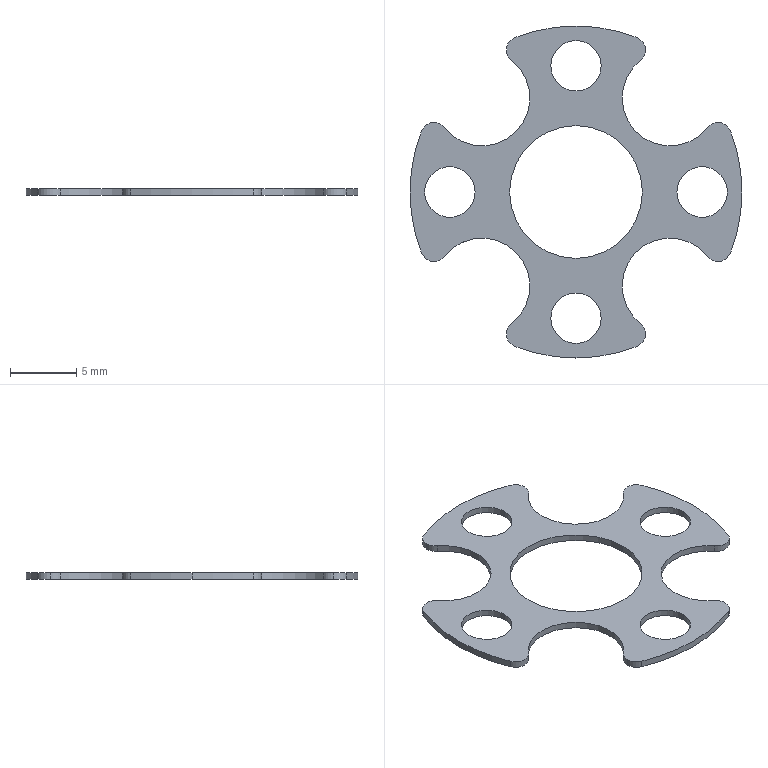Part | SolidWorks | features Extrusion 1 | 1 solid | 33 faces | box 25 x 25 x 0.5 mm | volume 107.561 mm3 | cylinder 31 | plane 2 | commonest cylinder face diameters 2 x10 3.8 x8 7.2 x6 25 x5 10 x2
STEP:
#1=CARTESIAN_POINT('',(-11.4,0.,0.5));
#2=VERTEX_POINT('',#1);
#3=CARTESIAN_POINT('',(-7.6,0.,0.5));
#4=VERTEX_POINT('',#3);
#5=CARTESIAN_POINT('',(-9.5,0.,0.5));
#6=DIRECTION('',(0.,0.,1.));
#7=DIRECTION('',(1.,0.,0.));
#8=AXIS2_PLACEMENT_3D('',#5,#6,#7);
#9=CIRCLE('',#8,1.9);
#10=EDGE_CURVE('',#2,#4,#9,.T.);
#11=ORIENTED_EDGE('',*,*,#10,.T.);
#12=CARTESIAN_POINT('',(-7.6,0.,0.));
#13=VERTEX_POINT('',#12);
#14=CARTESIAN_POINT('',(-7.6,0.,0.5));
#15=DIRECTION('',(0.,0.,-1.));
#16=VECTOR('',#15,1000.);
#17=LINE('',#14,#16);
#18=EDGE_CURVE('',#4,#13,#17,.T.);
#19=ORIENTED_EDGE('',*,*,#18,.T.);
#20=CARTESIAN_POINT('',(-11.4,0.,0.));
#21=VERTEX_POINT('',#20);
#22=CARTESIAN_POINT('',(-9.5,0.,0.));
#23=DIRECTION('',(0.,0.,1.));
#24=DIRECTION('',(1.,0.,0.));
#25=AXIS2_PLACEMENT_3D('',#22,#23,#24);
#26=CIRCLE('',#25,1.9);
#27=EDGE_CURVE('',#21,#13,#26,.T.);
#28=ORIENTED_EDGE('',*,*,#27,.F.);
#29=CARTESIAN_POINT('',(-11.4,0.,0.5));
#30=DIRECTION('',(0.,0.,-1.));
#31=VECTOR('',#30,1000.);
#32=LINE('',#29,#31);
#33=EDGE_CURVE('',#2,#21,#32,.T.);
#34=ORIENTED_EDGE('',*,*,#33,.F.);
#35=EDGE_LOOP('',(#11,#19,#28,#34));
#36=FACE_OUTER_BOUND('',#35,.T.);
#37=CARTESIAN_POINT('',(-9.5,0.,0.5));
#38=DIRECTION('',(0.,0.,-1.));
#39=DIRECTION('',(-1.,0.,0.));
#40=AXIS2_PLACEMENT_3D('',#37,#38,#39);
#41=CYLINDRICAL_SURFACE('',#40,1.9);
#42=ADVANCED_FACE('',(#36),#41,.F.);
#43=CARTESIAN_POINT('',(-1.9,-9.5,0.5));
#44=VERTEX_POINT('',#43);
#45=CARTESIAN_POINT('',(1.9,-9.5,0.5));
#46=VERTEX_POINT('',#45);
#47=CARTESIAN_POINT('',(0.,-9.5,0.5));
#48=DIRECTION('',(0.,0.,1.));
#49=DIRECTION('',(1.,0.,0.));
#50=AXIS2_PLACEMENT_3D('',#47,#48,#49);
#51=CIRCLE('',#50,1.9);
#52=EDGE_CURVE('',#44,#46,#51,.T.);
#53=ORIENTED_EDGE('',*,*,#52,.T.);
#54=CARTESIAN_POINT('',(1.9,-9.5,0.));
#55=VERTEX_POINT('',#54);
#56=CARTESIAN_POINT('',(1.9,-9.5,0.5));
#57=DIRECTION('',(0.,0.,-1.));
#58=VECTOR('',#57,1000.);
#59=LINE('',#56,#58);
#60=EDGE_CURVE('',#46,#55,#59,.T.);
#61=ORIENTED_EDGE('',*,*,#60,.T.);
#62=CARTESIAN_POINT('',(-1.9,-9.5,0.));
#63=VERTEX_POINT('',#62);
#64=CARTESIAN_POINT('',(0.,-9.5,0.));
#65=DIRECTION('',(0.,0.,1.));
#66=DIRECTION('',(1.,0.,0.));
#67=AXIS2_PLACEMENT_3D('',#64,#65,#66);
#68=CIRCLE('',#67,1.9);
#69=EDGE_CURVE('',#63,#55,#68,.T.);
#70=ORIENTED_EDGE('',*,*,#69,.F.);
#71=CARTESIAN_POINT('',(-1.9,-9.5,0.5));
#72=DIRECTION('',(0.,0.,-1.));
#73=VECTOR('',#72,1000.);
#74=LINE('',#71,#73);
#75=EDGE_CURVE('',#44,#63,#74,.T.);
#76=ORIENTED_EDGE('',*,*,#75,.F.);
#77=EDGE_LOOP('',(#53,#61,#70,#76));
#78=FACE_OUTER_BOUND('',#77,.T.);
#79=CARTESIAN_POINT('',(0.,-9.5,0.5));
#80=DIRECTION('',(0.,0.,-1.));
#81=DIRECTION('',(-1.,0.,0.));
#82=AXIS2_PLACEMENT_3D('',#79,#80,#81);
#83=CYLINDRICAL_SURFACE('',#82,1.9);
#84=ADVANCED_FACE('',(#78),#83,.F.);
#85=CARTESIAN_POINT('',(7.6,0.,0.5));
#86=VERTEX_POINT('',#85);
#87=CARTESIAN_POINT('',(11.4,0.,0.5));
#88=VERTEX_POINT('',#87);
#89=CARTESIAN_POINT('',(9.5,0.,0.5));
#90=DIRECTION('',(0.,0.,1.));
#91=DIRECTION('',(1.,0.,0.));
#92=AXIS2_PLACEMENT_3D('',#89,#90,#91);
#93=CIRCLE('',#92,1.9);
#94=EDGE_CURVE('',#86,#88,#93,.T.);
#95=ORIENTED_EDGE('',*,*,#94,.T.);
#96=CARTESIAN_POINT('',(11.4,0.,0.));
#97=VERTEX_POINT('',#96);
#98=CARTESIAN_POINT('',(11.4,0.,0.5));
#99=DIRECTION('',(0.,0.,-1.));
#100=VECTOR('',#99,1000.);
#101=LINE('',#98,#100);
#102=EDGE_CURVE('',#88,#97,#101,.T.);
#103=ORIENTED_EDGE('',*,*,#102,.T.);
#104=CARTESIAN_POINT('',(7.6,0.,0.));
#105=VERTEX_POINT('',#104);
#106=CARTESIAN_POINT('',(9.5,0.,0.));
#107=DIRECTION('',(0.,0.,1.));
#108=DIRECTION('',(1.,0.,0.));
#109=AXIS2_PLACEMENT_3D('',#106,#107,#108);
#110=CIRCLE('',#109,1.9);
#111=EDGE_CURVE('',#105,#97,#110,.T.);
#112=ORIENTED_EDGE('',*,*,#111,.F.);
#113=CARTESIAN_POINT('',(7.6,0.,0.5));
#114=DIRECTION('',(0.,0.,-1.));
#115=VECTOR('',#114,1000.);
#116=LINE('',#113,#115);
#117=EDGE_CURVE('',#86,#105,#116,.T.);
#118=ORIENTED_EDGE('',*,*,#117,.F.);
#119=EDGE_LOOP('',(#95,#103,#112,#118));
#120=FACE_OUTER_BOUND('',#119,.T.);
#121=CARTESIAN_POINT('',(9.5,0.,0.5));
#122=DIRECTION('',(0.,0.,-1.));
#123=DIRECTION('',(-1.,0.,0.));
#124=AXIS2_PLACEMENT_3D('',#121,#122,#123);
#125=CYLINDRICAL_SURFACE('',#124,1.9);
#126=ADVANCED_FACE('',(#120),#125,.F.);
#127=CARTESIAN_POINT('',(-5.,0.,0.5));
#128=VERTEX_POINT('',#127);
#129=CARTESIAN_POINT('',(5.,0.,0.5));
#130=VERTEX_POINT('',#129);
#131=CARTESIAN_POINT('',(0.,0.,0.5));
#132=DIRECTION('',(0.,0.,1.));
#133=DIRECTION('',(1.,0.,0.));
#134=AXIS2_PLACEMENT_3D('',#131,#132,#133);
#135=CIRCLE('',#134,5.);
#136=EDGE_CURVE('',#128,#130,#135,.T.);
#137=ORIENTED_EDGE('',*,*,#136,.T.);
#138=CARTESIAN_POINT('',(5.,0.,0.));
#139=VERTEX_POINT('',#138);
#140=CARTESIAN_POINT('',(5.,0.,0.5));
#141=DIRECTION('',(0.,0.,-1.));
#142=VECTOR('',#141,1000.);
#143=LINE('',#140,#142);
#144=EDGE_CURVE('',#130,#139,#143,.T.);
#145=ORIENTED_EDGE('',*,*,#144,.T.);
#146=CARTESIAN_POINT('',(-5.,0.,0.));
#147=VERTEX_POINT('',#146);
#148=CARTESIAN_POINT('',(0.,0.,0.));
#149=DIRECTION('',(0.,0.,1.));
#150=DIRECTION('',(1.,0.,0.));
#151=AXIS2_PLACEMENT_3D('',#148,#149,#150);
#152=CIRCLE('',#151,5.);
#153=EDGE_CURVE('',#147,#139,#152,.T.);
#154=ORIENTED_EDGE('',*,*,#153,.F.);
#155=CARTESIAN_POINT('',(-5.,0.,0.5));
#156=DIRECTION('',(0.,0.,-1.));
#157=VECTOR('',#156,1000.);
#158=LINE('',#155,#157);
#159=EDGE_CURVE('',#128,#147,#158,.T.);
#160=ORIENTED_EDGE('',*,*,#159,.F.);
#161=EDGE_LOOP('',(#137,#145,#154,#160));
#162=FACE_OUTER_BOUND('',#161,.T.);
#163=CARTESIAN_POINT('',(0.,0.,0.5));
#164=DIRECTION('',(0.,0.,-1.));
#165=DIRECTION('',(-1.,0.,0.));
#166=AXIS2_PLACEMENT_3D('',#163,#164,#165);
#167=CYLINDRICAL_SURFACE('',#166,5.);
#168=ADVANCED_FACE('',(#162),#167,.F.);
#169=CARTESIAN_POINT('',(-1.9,9.5,0.5));
#170=VERTEX_POINT('',#169);
#171=CARTESIAN_POINT('',(1.9,9.5,0.5));
#172=VERTEX_POINT('',#171);
#173=CARTESIAN_POINT('',(0.,9.5,0.5));
#174=DIRECTION('',(0.,0.,1.));
#175=DIRECTION('',(1.,0.,0.));
#176=AXIS2_PLACEMENT_3D('',#173,#174,#175);
#177=CIRCLE('',#176,1.9);
#178=EDGE_CURVE('',#170,#172,#177,.T.);
#179=ORIENTED_EDGE('',*,*,#178,.T.);
#180=CARTESIAN_POINT('',(1.9,9.5,0.));
#181=VERTEX_POINT('',#180);
#182=CARTESIAN_POINT('',(1.9,9.5,0.5));
#183=DIRECTION('',(0.,0.,-1.));
#184=VECTOR('',#183,1000.);
#185=LINE('',#182,#184);
#186=EDGE_CURVE('',#172,#181,#185,.T.);
#187=ORIENTED_EDGE('',*,*,#186,.T.);
#188=CARTESIAN_POINT('',(-1.9,9.5,0.));
#189=VERTEX_POINT('',#188);
#190=CARTESIAN_POINT('',(0.,9.5,0.));
#191=DIRECTION('',(0.,0.,1.));
#192=DIRECTION('',(1.,0.,0.));
#193=AXIS2_PLACEMENT_3D('',#190,#191,#192);
#194=CIRCLE('',#193,1.9);
#195=EDGE_CURVE('',#189,#181,#194,.T.);
#196=ORIENTED_EDGE('',*,*,#195,.F.);
#197=CARTESIAN_POINT('',(-1.9,9.5,0.5));
#198=DIRECTION('',(0.,0.,-1.));
#199=VECTOR('',#198,1000.);
#200=LINE('',#197,#199);
#201=EDGE_CURVE('',#170,#189,#200,.T.);
#202=ORIENTED_EDGE('',*,*,#201,.F.);
#203=EDGE_LOOP('',(#179,#187,#196,#202));
#204=FACE_OUTER_BOUND('',#203,.T.);
#205=CARTESIAN_POINT('',(0.,9.5,0.5));
#206=DIRECTION('',(0.,0.,-1.));
#207=DIRECTION('',(-1.,0.,0.));
#208=AXIS2_PLACEMENT_3D('',#205,#206,#207);
#209=CYLINDRICAL_SURFACE('',#208,1.9);
#210=ADVANCED_FACE('',(#204),#209,.F.);
#211=CARTESIAN_POINT('',(3.471,-7.071,0.5));
#212=VERTEX_POINT('',#211);
#213=CARTESIAN_POINT('',(9.905,-4.851,0.5));
#214=VERTEX_POINT('',#213);
#215=CARTESIAN_POINT('',(7.071,-7.071,0.5));
#216=DIRECTION('',(0.,0.,-1.));
#217=DIRECTION('',(-1.,0.,0.));
#218=AXIS2_PLACEMENT_3D('',#215,#216,#217);
#219=CIRCLE('',#218,3.6);
#220=EDGE_CURVE('',#212,#214,#219,.T.);
#221=ORIENTED_EDGE('',*,*,#220,.F.);
#222=CARTESIAN_POINT('',(3.471,-7.071,0.));
#223=VERTEX_POINT('',#222);
#224=CARTESIAN_POINT('',(3.471,-7.071,0.5));
#225=DIRECTION('',(0.,0.,-1.));
#226=VECTOR('',#225,1000.);
#227=LINE('',#224,#226);
#228=EDGE_CURVE('',#212,#223,#227,.T.);
#229=ORIENTED_EDGE('',*,*,#228,.T.);
#230=CARTESIAN_POINT('',(9.905,-4.851,0.));
#231=VERTEX_POINT('',#230);
#232=CARTESIAN_POINT('',(7.071,-7.071,0.));
#233=DIRECTION('',(0.,0.,-1.));
#234=DIRECTION('',(-1.,0.,0.));
#235=AXIS2_PLACEMENT_3D('',#232,#233,#234);
#236=CIRCLE('',#235,3.6);
#237=EDGE_CURVE('',#223,#231,#236,.T.);
#238=ORIENTED_EDGE('',*,*,#237,.T.);
#239=CARTESIAN_POINT('',(9.905,-4.851,0.5));
#240=DIRECTION('',(0.,0.,-1.));
#241=VECTOR('',#240,1000.);
#242=LINE('',#239,#241);
#243=EDGE_CURVE('',#214,#231,#242,.T.);
#244=ORIENTED_EDGE('',*,*,#243,.F.);
#245=EDGE_LOOP('',(#221,#229,#238,#244));
#246=FACE_OUTER_BOUND('',#245,.T.);
#247=CARTESIAN_POINT('',(7.071,-7.071,0.5));
#248=DIRECTION('',(0.,0.,-1.));
#249=DIRECTION('',(-1.,0.,0.));
#250=AXIS2_PLACEMENT_3D('',#247,#248,#249);
#251=CYLINDRICAL_SURFACE('',#250,3.6);
#252=ADVANCED_FACE('',(#246),#251,.F.);
#253=CARTESIAN_POINT('',(-5.234,-10.692,0.5));
#254=VERTEX_POINT('',#253);
#255=CARTESIAN_POINT('',(-4.602,-11.622,0.5));
#256=VERTEX_POINT('',#255);
#257=CARTESIAN_POINT('',(-4.234,-10.692,0.5));
#258=DIRECTION('',(0.,0.,1.));
#259=DIRECTION('',(1.,0.,0.));
#260=AXIS2_PLACEMENT_3D('',#257,#258,#259);
#261=CIRCLE('',#260,1.);
#262=EDGE_CURVE('',#254,#256,#261,.T.);
#263=ORIENTED_EDGE('',*,*,#262,.F.);
#264=CARTESIAN_POINT('',(-5.234,-10.692,0.));
#265=VERTEX_POINT('',#264);
#266=CARTESIAN_POINT('',(-5.234,-10.692,0.5));
#267=DIRECTION('',(0.,0.,-1.));
#268=VECTOR('',#267,1000.);
#269=LINE('',#266,#268);
#270=EDGE_CURVE('',#254,#265,#269,.T.);
#271=ORIENTED_EDGE('',*,*,#270,.T.);
#272=CARTESIAN_POINT('',(-4.602,-11.622,0.));
#273=VERTEX_POINT('',#272);
#274=CARTESIAN_POINT('',(-4.234,-10.692,0.));
#275=DIRECTION('',(0.,0.,1.));
#276=DIRECTION('',(1.,0.,0.));
#277=AXIS2_PLACEMENT_3D('',#274,#275,#276);
#278=CIRCLE('',#277,1.);
#279=EDGE_CURVE('',#265,#273,#278,.T.);
#280=ORIENTED_EDGE('',*,*,#279,.T.);
#281=CARTESIAN_POINT('',(-4.602,-11.622,0.5));
#282=DIRECTION('',(0.,0.,-1.));
#283=VECTOR('',#282,1000.);
#284=LINE('',#281,#283);
#285=EDGE_CURVE('',#256,#273,#284,.T.);
#286=ORIENTED_EDGE('',*,*,#285,.F.);
#287=EDGE_LOOP('',(#263,#271,#280,#286));
#288=FACE_OUTER_BOUND('',#287,.T.);
#289=CARTESIAN_POINT('',(-4.234,-10.692,0.5));
#290=DIRECTION('',(0.,0.,-1.));
#291=DIRECTION('',(-1.,0.,0.));
#292=AXIS2_PLACEMENT_3D('',#289,#290,#291);
#293=CYLINDRICAL_SURFACE('',#292,1.);
#294=ADVANCED_FACE('',(#288),#293,.T.);
#295=CARTESIAN_POINT('',(-12.5,0.,0.5));
#296=VERTEX_POINT('',#295);
#297=CARTESIAN_POINT('',(-11.622,-4.602,0.5));
#298=VERTEX_POINT('',#297);
#299=CARTESIAN_POINT('',(0.,0.,0.5));
#300=DIRECTION('',(0.,0.,1.));
#301=DIRECTION('',(1.,0.,0.));
#302=AXIS2_PLACEMENT_3D('',#299,#300,#301);
#303=CIRCLE('',#302,12.5);
#304=EDGE_CURVE('',#296,#298,#303,.T.);
#305=ORIENTED_EDGE('',*,*,#304,.F.);
#306=CARTESIAN_POINT('',(-12.5,0.,0.));
#307=VERTEX_POINT('',#306);
#308=CARTESIAN_POINT('',(-12.5,0.,0.5));
#309=DIRECTION('',(0.,0.,-1.));
#310=VECTOR('',#309,1000.);
#311=LINE('',#308,#310);
#312=EDGE_CURVE('',#296,#307,#311,.T.);
#313=ORIENTED_EDGE('',*,*,#312,.T.);
#314=CARTESIAN_POINT('',(-11.622,-4.602,0.));
#315=VERTEX_POINT('',#314);
#316=CARTESIAN_POINT('',(0.,0.,0.));
#317=DIRECTION('',(0.,0.,1.));
#318=DIRECTION('',(1.,0.,0.));
#319=AXIS2_PLACEMENT_3D('',#316,#317,#318);
#320=CIRCLE('',#319,12.5);
#321=EDGE_CURVE('',#307,#315,#320,.T.);
#322=ORIENTED_EDGE('',*,*,#321,.T.);
#323=CARTESIAN_POINT('',(-11.622,-4.602,0.5));
#324=DIRECTION('',(0.,0.,-1.));
#325=VECTOR('',#324,1000.);
#326=LINE('',#323,#325);
#327=EDGE_CURVE('',#298,#315,#326,.T.);
#328=ORIENTED_EDGE('',*,*,#327,.F.);
#329=EDGE_LOOP('',(#305,#313,#322,#328));
#330=FACE_OUTER_BOUND('',#329,.T.);
#331=CARTESIAN_POINT('',(0.,0.,0.5));
#332=DIRECTION('',(0.,0.,-1.));
#333=DIRECTION('',(-1.,0.,0.));
#334=AXIS2_PLACEMENT_3D('',#331,#332,#333);
#335=CYLINDRICAL_SURFACE('',#334,12.5);
#336=ADVANCED_FACE('',(#330),#335,.T.);
#337=CARTESIAN_POINT('',(-5.234,10.692,0.5));
#338=VERTEX_POINT('',#337);
#339=CARTESIAN_POINT('',(-4.851,9.905,0.5));
#340=VERTEX_POINT('',#339);
#341=CARTESIAN_POINT('',(-4.234,10.692,0.5));
#342=DIRECTION('',(0.,0.,1.));
#343=DIRECTION('',(-1.,0.,0.));
#344=AXIS2_PLACEMENT_3D('',#341,#342,#343);
#345=CIRCLE('',#344,1.);
#346=EDGE_CURVE('',#338,#340,#345,.T.);
#347=ORIENTED_EDGE('',*,*,#346,.F.);
#348=CARTESIAN_POINT('',(-5.234,10.692,0.));
#349=VERTEX_POINT('',#348);
#350=CARTESIAN_POINT('',(-5.234,10.692,0.5));
#351=DIRECTION('',(0.,0.,-1.));
#352=VECTOR('',#351,1000.);
#353=LINE('',#350,#352);
#354=EDGE_CURVE('',#338,#349,#353,.T.);
#355=ORIENTED_EDGE('',*,*,#354,.T.);
#356=CARTESIAN_POINT('',(-4.851,9.905,0.));
#357=VERTEX_POINT('',#356);
#358=CARTESIAN_POINT('',(-4.234,10.692,0.));
#359=DIRECTION('',(0.,0.,1.));
#360=DIRECTION('',(-1.,0.,0.));
#361=AXIS2_PLACEMENT_3D('',#358,#359,#360);
#362=CIRCLE('',#361,1.);
#363=EDGE_CURVE('',#349,#357,#362,.T.);
#364=ORIENTED_EDGE('',*,*,#363,.T.);
#365=CARTESIAN_POINT('',(-4.851,9.905,0.5));
#366=DIRECTION('',(0.,0.,-1.));
#367=VECTOR('',#366,1000.);
#368=LINE('',#365,#367);
#369=EDGE_CURVE('',#340,#357,#368,.T.);
#370=ORIENTED_EDGE('',*,*,#369,.F.);
#371=EDGE_LOOP('',(#347,#355,#364,#370));
#372=FACE_OUTER_BOUND('',#371,.T.);
#373=CARTESIAN_POINT('',(-4.234,10.692,0.5));
#374=DIRECTION('',(0.,0.,-1.));
#375=DIRECTION('',(-1.,0.,0.));
#376=AXIS2_PLACEMENT_3D('',#373,#374,#375);
#377=CYLINDRICAL_SURFACE('',#376,1.);
#378=ADVANCED_FACE('',(#372),#377,.T.);
#379=CARTESIAN_POINT('',(3.471,7.071,0.5));
#380=VERTEX_POINT('',#379);
#381=CARTESIAN_POINT('',(4.851,9.905,0.5));
#382=VERTEX_POINT('',#381);
#383=CARTESIAN_POINT('',(7.071,7.071,0.5));
#384=DIRECTION('',(0.,0.,-1.));
#385=DIRECTION('',(1.,0.,0.));
#386=AXIS2_PLACEMENT_3D('',#383,#384,#385);
#387=CIRCLE('',#386,3.6);
#388=EDGE_CURVE('',#380,#382,#387,.T.);
#389=ORIENTED_EDGE('',*,*,#388,.F.);
#390=CARTESIAN_POINT('',(3.471,7.071,0.));
#391=VERTEX_POINT('',#390);
#392=CARTESIAN_POINT('',(3.471,7.071,0.5));
#393=DIRECTION('',(0.,0.,-1.));
#394=VECTOR('',#393,1000.);
#395=LINE('',#392,#394);
#396=EDGE_CURVE('',#380,#391,#395,.T.);
#397=ORIENTED_EDGE('',*,*,#396,.T.);
#398=CARTESIAN_POINT('',(4.851,9.905,0.));
#399=VERTEX_POINT('',#398);
#400=CARTESIAN_POINT('',(7.071,7.071,0.));
#401=DIRECTION('',(0.,0.,-1.));
#402=DIRECTION('',(1.,0.,0.));
#403=AXIS2_PLACEMENT_3D('',#400,#401,#402);
#404=CIRCLE('',#403,3.6);
#405=EDGE_CURVE('',#391,#399,#404,.T.);
#406=ORIENTED_EDGE('',*,*,#405,.T.);
#407=CARTESIAN_POINT('',(4.851,9.905,0.5));
#408=DIRECTION('',(0.,0.,-1.));
#409=VECTOR('',#408,1000.);
#410=LINE('',#407,#409);
#411=EDGE_CURVE('',#382,#399,#410,.T.);
#412=ORIENTED_EDGE('',*,*,#411,.F.);
#413=EDGE_LOOP('',(#389,#397,#406,#412));
#414=FACE_OUTER_BOUND('',#413,.T.);
#415=CARTESIAN_POINT('',(7.071,7.071,0.5));
#416=DIRECTION('',(0.,0.,-1.));
#417=DIRECTION('',(-1.,0.,0.));
#418=AXIS2_PLACEMENT_3D('',#415,#416,#417);
#419=CYLINDRICAL_SURFACE('',#418,3.6);
#420=ADVANCED_FACE('',(#414),#419,.F.);
#421=ORIENTED_EDGE('',*,*,#52,.F.);
#422=CARTESIAN_POINT('',(0.,-9.5,0.5));
#423=DIRECTION('',(0.,0.,1.));
#424=DIRECTION('',(1.,0.,0.));
#425=AXIS2_PLACEMENT_3D('',#422,#423,#424);
#426=CIRCLE('',#425,1.9);
#427=EDGE_CURVE('',#46,#44,#426,.T.);
#428=ORIENTED_EDGE('',*,*,#427,.F.);
#429=EDGE_LOOP('',(#421,#428));
#430=FACE_BOUND('',#429,.T.);
#431=ORIENTED_EDGE('',*,*,#136,.F.);
#432=CARTESIAN_POINT('',(0.,0.,0.5));
#433=DIRECTION('',(0.,0.,1.));
#434=DIRECTION('',(1.,0.,0.));
#435=AXIS2_PLACEMENT_3D('',#432,#433,#434);
#436=CIRCLE('',#435,5.);
#437=EDGE_CURVE('',#130,#128,#436,.T.);
#438=ORIENTED_EDGE('',*,*,#437,.F.);
#439=EDGE_LOOP('',(#431,#438));
#440=FACE_BOUND('',#439,.T.);
#441=CARTESIAN_POINT('',(11.622,-4.602,0.5));
#442=VERTEX_POINT('',#441);
#443=CARTESIAN_POINT('',(10.692,-4.234,0.5));
#444=DIRECTION('',(0.,0.,1.));
#445=DIRECTION('',(1.,0.,0.));
#446=AXIS2_PLACEMENT_3D('',#443,#444,#445);
#447=CIRCLE('',#446,1.);
#448=EDGE_CURVE('',#214,#442,#447,.T.);
#449=ORIENTED_EDGE('',*,*,#448,.T.);
#450=CARTESIAN_POINT('',(11.622,4.602,0.5));
#451=VERTEX_POINT('',#450);
#452=CARTESIAN_POINT('',(0.,0.,0.5));
#453=DIRECTION('',(0.,0.,1.));
#454=DIRECTION('',(1.,0.,0.));
#455=AXIS2_PLACEMENT_3D('',#452,#453,#454);
#456=CIRCLE('',#455,12.5);
#457=EDGE_CURVE('',#442,#451,#456,.T.);
#458=ORIENTED_EDGE('',*,*,#457,.T.);
#459=CARTESIAN_POINT('',(9.905,4.851,0.5));
#460=VERTEX_POINT('',#459);
#461=CARTESIAN_POINT('',(10.692,4.234,0.5));
#462=DIRECTION('',(0.,0.,1.));
#463=DIRECTION('',(-1.,0.,0.));
#464=AXIS2_PLACEMENT_3D('',#461,#462,#463);
#465=CIRCLE('',#464,1.);
#466=EDGE_CURVE('',#451,#460,#465,.T.);
#467=ORIENTED_EDGE('',*,*,#466,.T.);
#468=CARTESIAN_POINT('',(7.071,7.071,0.5));
#469=DIRECTION('',(0.,0.,-1.));
#470=DIRECTION('',(1.,0.,0.));
#471=AXIS2_PLACEMENT_3D('',#468,#469,#470);
#472=CIRCLE('',#471,3.6);
#473=EDGE_CURVE('',#460,#380,#472,.T.);
#474=ORIENTED_EDGE('',*,*,#473,.T.);
#475=ORIENTED_EDGE('',*,*,#388,.T.);
#476=CARTESIAN_POINT('',(4.602,11.622,0.5));
#477=VERTEX_POINT('',#476);
#478=CARTESIAN_POINT('',(4.234,10.692,0.5));
#479=DIRECTION('',(0.,0.,1.));
#480=DIRECTION('',(1.,0.,0.));
#481=AXIS2_PLACEMENT_3D('',#478,#479,#480);
#482=CIRCLE('',#481,1.);
#483=EDGE_CURVE('',#382,#477,#482,.T.);
#484=ORIENTED_EDGE('',*,*,#483,.T.);
#485=CARTESIAN_POINT('',(-4.602,11.622,0.5));
#486=VERTEX_POINT('',#485);
#487=CARTESIAN_POINT('',(0.,0.,0.5));
#488=DIRECTION('',(0.,0.,1.));
#489=DIRECTION('',(1.,0.,0.));
#490=AXIS2_PLACEMENT_3D('',#487,#488,#489);
#491=CIRCLE('',#490,12.5);
#492=EDGE_CURVE('',#477,#486,#491,.T.);
#493=ORIENTED_EDGE('',*,*,#492,.T.);
#494=CARTESIAN_POINT('',(-4.234,10.692,0.5));
#495=DIRECTION('',(0.,0.,1.));
#496=DIRECTION('',(-1.,0.,0.));
#497=AXIS2_PLACEMENT_3D('',#494,#495,#496);
#498=CIRCLE('',#497,1.);
#499=EDGE_CURVE('',#486,#338,#498,.T.);
#500=ORIENTED_EDGE('',*,*,#499,.T.);
#501=ORIENTED_EDGE('',*,*,#346,.T.);
#502=CARTESIAN_POINT('',(-9.905,4.851,0.5));
#503=VERTEX_POINT('',#502);
#504=CARTESIAN_POINT('',(-7.071,7.071,0.5));
#505=DIRECTION('',(0.,0.,-1.));
#506=DIRECTION('',(-1.,0.,0.));
#507=AXIS2_PLACEMENT_3D('',#504,#505,#506);
#508=CIRCLE('',#507,3.6);
#509=EDGE_CURVE('',#340,#503,#508,.T.);
#510=ORIENTED_EDGE('',*,*,#509,.T.);
#511=CARTESIAN_POINT('',(-11.622,4.602,0.5));
#512=VERTEX_POINT('',#511);
#513=CARTESIAN_POINT('',(-10.692,4.234,0.5));
#514=DIRECTION('',(0.,0.,1.));
#515=DIRECTION('',(1.,0.,0.));
#516=AXIS2_PLACEMENT_3D('',#513,#514,#515);
#517=CIRCLE('',#516,1.);
#518=EDGE_CURVE('',#503,#512,#517,.T.);
#519=ORIENTED_EDGE('',*,*,#518,.T.);
#520=CARTESIAN_POINT('',(0.,0.,0.5));
#521=DIRECTION('',(0.,0.,1.));
#522=DIRECTION('',(1.,0.,0.));
#523=AXIS2_PLACEMENT_3D('',#520,#521,#522);
#524=CIRCLE('',#523,12.5);
#525=EDGE_CURVE('',#512,#296,#524,.T.);
#526=ORIENTED_EDGE('',*,*,#525,.T.);
#527=ORIENTED_EDGE('',*,*,#304,.T.);
#528=CARTESIAN_POINT('',(-9.905,-4.851,0.5));
#529=VERTEX_POINT('',#528);
#530=CARTESIAN_POINT('',(-10.692,-4.234,0.5));
#531=DIRECTION('',(0.,0.,1.));
#532=DIRECTION('',(-1.,0.,0.));
#533=AXIS2_PLACEMENT_3D('',#530,#531,#532);
#534=CIRCLE('',#533,1.);
#535=EDGE_CURVE('',#298,#529,#534,.T.);
#536=ORIENTED_EDGE('',*,*,#535,.T.);
#537=CARTESIAN_POINT('',(-4.851,-9.905,0.5));
#538=VERTEX_POINT('',#537);
#539=CARTESIAN_POINT('',(-7.071,-7.071,0.5));
#540=DIRECTION('',(0.,0.,-1.));
#541=DIRECTION('',(1.,0.,0.));
#542=AXIS2_PLACEMENT_3D('',#539,#540,#541);
#543=CIRCLE('',#542,3.6);
#544=EDGE_CURVE('',#529,#538,#543,.T.);
#545=ORIENTED_EDGE('',*,*,#544,.T.);
#546=CARTESIAN_POINT('',(-4.234,-10.692,0.5));
#547=DIRECTION('',(0.,0.,1.));
#548=DIRECTION('',(1.,0.,0.));
#549=AXIS2_PLACEMENT_3D('',#546,#547,#548);
#550=CIRCLE('',#549,1.);
#551=EDGE_CURVE('',#538,#254,#550,.T.);
#552=ORIENTED_EDGE('',*,*,#551,.T.);
#553=ORIENTED_EDGE('',*,*,#262,.T.);
#554=CARTESIAN_POINT('',(4.602,-11.622,0.5));
#555=VERTEX_POINT('',#554);
#556=CARTESIAN_POINT('',(0.,0.,0.5));
#557=DIRECTION('',(0.,0.,1.));
#558=DIRECTION('',(1.,0.,0.));
#559=AXIS2_PLACEMENT_3D('',#556,#557,#558);
#560=CIRCLE('',#559,12.5);
#561=EDGE_CURVE('',#256,#555,#560,.T.);
#562=ORIENTED_EDGE('',*,*,#561,.T.);
#563=CARTESIAN_POINT('',(4.851,-9.905,0.5));
#564=VERTEX_POINT('',#563);
#565=CARTESIAN_POINT('',(4.234,-10.692,0.5));
#566=DIRECTION('',(0.,0.,1.));
#567=DIRECTION('',(-1.,0.,0.));
#568=AXIS2_PLACEMENT_3D('',#565,#566,#567);
#569=CIRCLE('',#568,1.);
#570=EDGE_CURVE('',#555,#564,#569,.T.);
#571=ORIENTED_EDGE('',*,*,#570,.T.);
#572=CARTESIAN_POINT('',(7.071,-7.071,0.5));
#573=DIRECTION('',(0.,0.,-1.));
#574=DIRECTION('',(-1.,0.,0.));
#575=AXIS2_PLACEMENT_3D('',#572,#573,#574);
#576=CIRCLE('',#575,3.6);
#577=EDGE_CURVE('',#564,#212,#576,.T.);
#578=ORIENTED_EDGE('',*,*,#577,.T.);
#579=ORIENTED_EDGE('',*,*,#220,.T.);
#580=EDGE_LOOP('',(#449,#458,#467,#474,#475,#484,#493,#500,#501,#510,#519,#526,#527,#536,#545,#552,#553,#562,#571,#578,#579));
#581=FACE_OUTER_BOUND('',#580,.T.);
#582=ORIENTED_EDGE('',*,*,#178,.F.);
#583=CARTESIAN_POINT('',(0.,9.5,0.5));
#584=DIRECTION('',(0.,0.,1.));
#585=DIRECTION('',(1.,0.,0.));
#586=AXIS2_PLACEMENT_3D('',#583,#584,#585);
#587=CIRCLE('',#586,1.9);
#588=EDGE_CURVE('',#172,#170,#587,.T.);
#589=ORIENTED_EDGE('',*,*,#588,.F.);
#590=EDGE_LOOP('',(#582,#589));
#591=FACE_BOUND('',#590,.T.);
#592=ORIENTED_EDGE('',*,*,#94,.F.);
#593=CARTESIAN_POINT('',(9.5,0.,0.5));
#594=DIRECTION('',(0.,0.,1.));
#595=DIRECTION('',(1.,0.,0.));
#596=AXIS2_PLACEMENT_3D('',#593,#594,#595);
#597=CIRCLE('',#596,1.9);
#598=EDGE_CURVE('',#88,#86,#597,.T.);
#599=ORIENTED_EDGE('',*,*,#598,.F.);
#600=EDGE_LOOP('',(#592,#599));
#601=FACE_BOUND('',#600,.T.);
#602=ORIENTED_EDGE('',*,*,#10,.F.);
#603=CARTESIAN_POINT('',(-9.5,0.,0.5));
#604=DIRECTION('',(0.,0.,1.));
#605=DIRECTION('',(1.,0.,0.));
#606=AXIS2_PLACEMENT_3D('',#603,#604,#605);
#607=CIRCLE('',#606,1.9);
#608=EDGE_CURVE('',#4,#2,#607,.T.);
#609=ORIENTED_EDGE('',*,*,#608,.F.);
#610=EDGE_LOOP('',(#602,#609));
#611=FACE_BOUND('',#610,.T.);
#612=CARTESIAN_POINT('',(5.346,-2.117,0.5));
#613=DIRECTION('',(0.,0.,1.));
#614=DIRECTION('',(1.,0.,0.));
#615=AXIS2_PLACEMENT_3D('',#612,#613,#614);
#616=PLANE('',#615);
#617=ADVANCED_FACE('',(#430,#440,#581,#591,#601,#611),#616,.T.);
#618=CARTESIAN_POINT('',(11.622,-4.602,0.));
#619=VERTEX_POINT('',#618);
#620=CARTESIAN_POINT('',(10.692,-4.234,0.));
#621=DIRECTION('',(0.,0.,1.));
#622=DIRECTION('',(1.,0.,0.));
#623=AXIS2_PLACEMENT_3D('',#620,#621,#622);
#624=CIRCLE('',#623,1.);
#625=EDGE_CURVE('',#231,#619,#624,.T.);
#626=ORIENTED_EDGE('',*,*,#625,.F.);
#627=ORIENTED_EDGE('',*,*,#237,.F.);
#628=CARTESIAN_POINT('',(4.851,-9.905,0.));
#629=VERTEX_POINT('',#628);
#630=CARTESIAN_POINT('',(7.071,-7.071,0.));
#631=DIRECTION('',(0.,0.,-1.));
#632=DIRECTION('',(-1.,0.,0.));
#633=AXIS2_PLACEMENT_3D('',#630,#631,#632);
#634=CIRCLE('',#633,3.6);
#635=EDGE_CURVE('',#629,#223,#634,.T.);
#636=ORIENTED_EDGE('',*,*,#635,.F.);
#637=CARTESIAN_POINT('',(4.602,-11.622,0.));
#638=VERTEX_POINT('',#637);
#639=CARTESIAN_POINT('',(4.234,-10.692,0.));
#640=DIRECTION('',(0.,0.,1.));
#641=DIRECTION('',(-1.,0.,0.));
#642=AXIS2_PLACEMENT_3D('',#639,#640,#641);
#643=CIRCLE('',#642,1.);
#644=EDGE_CURVE('',#638,#629,#643,.T.);
#645=ORIENTED_EDGE('',*,*,#644,.F.);
#646=CARTESIAN_POINT('',(0.,0.,0.));
#647=DIRECTION('',(0.,0.,1.));
#648=DIRECTION('',(1.,0.,0.));
#649=AXIS2_PLACEMENT_3D('',#646,#647,#648);
#650=CIRCLE('',#649,12.5);
#651=EDGE_CURVE('',#273,#638,#650,.T.);
#652=ORIENTED_EDGE('',*,*,#651,.F.);
#653=ORIENTED_EDGE('',*,*,#279,.F.);
#654=CARTESIAN_POINT('',(-4.851,-9.905,0.));
#655=VERTEX_POINT('',#654);
#656=CARTESIAN_POINT('',(-4.234,-10.692,0.));
#657=DIRECTION('',(0.,0.,1.));
#658=DIRECTION('',(1.,0.,0.));
#659=AXIS2_PLACEMENT_3D('',#656,#657,#658);
#660=CIRCLE('',#659,1.);
#661=EDGE_CURVE('',#655,#265,#660,.T.);
#662=ORIENTED_EDGE('',*,*,#661,.F.);
#663=CARTESIAN_POINT('',(-9.905,-4.851,0.));
#664=VERTEX_POINT('',#663);
#665=CARTESIAN_POINT('',(-7.071,-7.071,0.));
#666=DIRECTION('',(0.,0.,-1.));
#667=DIRECTION('',(1.,0.,0.));
#668=AXIS2_PLACEMENT_3D('',#665,#666,#667);
#669=CIRCLE('',#668,3.6);
#670=EDGE_CURVE('',#664,#655,#669,.T.);
#671=ORIENTED_EDGE('',*,*,#670,.F.);
#672=CARTESIAN_POINT('',(-10.692,-4.234,0.));
#673=DIRECTION('',(0.,0.,1.));
#674=DIRECTION('',(-1.,0.,0.));
#675=AXIS2_PLACEMENT_3D('',#672,#673,#674);
#676=CIRCLE('',#675,1.);
#677=EDGE_CURVE('',#315,#664,#676,.T.);
#678=ORIENTED_EDGE('',*,*,#677,.F.);
#679=ORIENTED_EDGE('',*,*,#321,.F.);
#680=CARTESIAN_POINT('',(-11.622,4.602,0.));
#681=VERTEX_POINT('',#680);
#682=CARTESIAN_POINT('',(0.,0.,0.));
#683=DIRECTION('',(0.,0.,1.));
#684=DIRECTION('',(1.,0.,0.));
#685=AXIS2_PLACEMENT_3D('',#682,#683,#684);
#686=CIRCLE('',#685,12.5);
#687=EDGE_CURVE('',#681,#307,#686,.T.);
#688=ORIENTED_EDGE('',*,*,#687,.F.);
#689=CARTESIAN_POINT('',(-9.905,4.851,0.));
#690=VERTEX_POINT('',#689);
#691=CARTESIAN_POINT('',(-10.692,4.234,0.));
#692=DIRECTION('',(0.,0.,1.));
#693=DIRECTION('',(1.,0.,0.));
#694=AXIS2_PLACEMENT_3D('',#691,#692,#693);
#695=CIRCLE('',#694,1.);
#696=EDGE_CURVE('',#690,#681,#695,.T.);
#697=ORIENTED_EDGE('',*,*,#696,.F.);
#698=CARTESIAN_POINT('',(-7.071,7.071,0.));
#699=DIRECTION('',(0.,0.,-1.));
#700=DIRECTION('',(-1.,0.,0.));
#701=AXIS2_PLACEMENT_3D('',#698,#699,#700);
#702=CIRCLE('',#701,3.6);
#703=EDGE_CURVE('',#357,#690,#702,.T.);
#704=ORIENTED_EDGE('',*,*,#703,.F.);
#705=ORIENTED_EDGE('',*,*,#363,.F.);
#706=CARTESIAN_POINT('',(-4.602,11.622,0.));
#707=VERTEX_POINT('',#706);
#708=CARTESIAN_POINT('',(-4.234,10.692,0.));
#709=DIRECTION('',(0.,0.,1.));
#710=DIRECTION('',(-1.,0.,0.));
#711=AXIS2_PLACEMENT_3D('',#708,#709,#710);
#712=CIRCLE('',#711,1.);
#713=EDGE_CURVE('',#707,#349,#712,.T.);
#714=ORIENTED_EDGE('',*,*,#713,.F.);
#715=CARTESIAN_POINT('',(4.602,11.622,0.));
#716=VERTEX_POINT('',#715);
#717=CARTESIAN_POINT('',(0.,0.,0.));
#718=DIRECTION('',(0.,0.,1.));
#719=DIRECTION('',(1.,0.,0.));
#720=AXIS2_PLACEMENT_3D('',#717,#718,#719);
#721=CIRCLE('',#720,12.5);
#722=EDGE_CURVE('',#716,#707,#721,.T.);
#723=ORIENTED_EDGE('',*,*,#722,.F.);
#724=CARTESIAN_POINT('',(4.234,10.692,0.));
#725=DIRECTION('',(0.,0.,1.));
#726=DIRECTION('',(1.,0.,0.));
#727=AXIS2_PLACEMENT_3D('',#724,#725,#726);
#728=CIRCLE('',#727,1.);
#729=EDGE_CURVE('',#399,#716,#728,.T.);
#730=ORIENTED_EDGE('',*,*,#729,.F.);
#731=ORIENTED_EDGE('',*,*,#405,.F.);
#732=CARTESIAN_POINT('',(9.905,4.851,0.));
#733=VERTEX_POINT('',#732);
#734=CARTESIAN_POINT('',(7.071,7.071,0.));
#735=DIRECTION('',(0.,0.,-1.));
#736=DIRECTION('',(1.,0.,0.));
#737=AXIS2_PLACEMENT_3D('',#734,#735,#736);
#738=CIRCLE('',#737,3.6);
#739=EDGE_CURVE('',#733,#391,#738,.T.);
#740=ORIENTED_EDGE('',*,*,#739,.F.);
#741=CARTESIAN_POINT('',(11.622,4.602,0.));
#742=VERTEX_POINT('',#741);
#743=CARTESIAN_POINT('',(10.692,4.234,0.));
#744=DIRECTION('',(0.,0.,1.));
#745=DIRECTION('',(-1.,0.,0.));
#746=AXIS2_PLACEMENT_3D('',#743,#744,#745);
#747=CIRCLE('',#746,1.);
#748=EDGE_CURVE('',#742,#733,#747,.T.);
#749=ORIENTED_EDGE('',*,*,#748,.F.);
#750=CARTESIAN_POINT('',(0.,0.,0.));
#751=DIRECTION('',(0.,0.,1.));
#752=DIRECTION('',(1.,0.,0.));
#753=AXIS2_PLACEMENT_3D('',#750,#751,#752);
#754=CIRCLE('',#753,12.5);
#755=EDGE_CURVE('',#619,#742,#754,.T.);
#756=ORIENTED_EDGE('',*,*,#755,.F.);
#757=EDGE_LOOP('',(#626,#627,#636,#645,#652,#653,#662,#671,#678,#679,#688,#697,#704,#705,#714,#723,#730,#731,#740,#749,#756));
#758=FACE_OUTER_BOUND('',#757,.T.);
#759=ORIENTED_EDGE('',*,*,#195,.T.);
#760=CARTESIAN_POINT('',(0.,9.5,0.));
#761=DIRECTION('',(0.,0.,1.));
#762=DIRECTION('',(1.,0.,0.));
#763=AXIS2_PLACEMENT_3D('',#760,#761,#762);
#764=CIRCLE('',#763,1.9);
#765=EDGE_CURVE('',#181,#189,#764,.T.);
#766=ORIENTED_EDGE('',*,*,#765,.T.);
#767=EDGE_LOOP('',(#759,#766));
#768=FACE_BOUND('',#767,.T.);
#769=ORIENTED_EDGE('',*,*,#153,.T.);
#770=CARTESIAN_POINT('',(0.,0.,0.));
#771=DIRECTION('',(0.,0.,1.));
#772=DIRECTION('',(1.,0.,0.));
#773=AXIS2_PLACEMENT_3D('',#770,#771,#772);
#774=CIRCLE('',#773,5.);
#775=EDGE_CURVE('',#139,#147,#774,.T.);
#776=ORIENTED_EDGE('',*,*,#775,.T.);
#777=EDGE_LOOP('',(#769,#776));
#778=FACE_BOUND('',#777,.T.);
#779=ORIENTED_EDGE('',*,*,#111,.T.);
#780=CARTESIAN_POINT('',(9.5,0.,0.));
#781=DIRECTION('',(0.,0.,1.));
#782=DIRECTION('',(1.,0.,0.));
#783=AXIS2_PLACEMENT_3D('',#780,#781,#782);
#784=CIRCLE('',#783,1.9);
#785=EDGE_CURVE('',#97,#105,#784,.T.);
#786=ORIENTED_EDGE('',*,*,#785,.T.);
#787=EDGE_LOOP('',(#779,#786));
#788=FACE_BOUND('',#787,.T.);
#789=ORIENTED_EDGE('',*,*,#69,.T.);
#790=CARTESIAN_POINT('',(0.,-9.5,0.));
#791=DIRECTION('',(0.,0.,1.));
#792=DIRECTION('',(1.,0.,0.));
#793=AXIS2_PLACEMENT_3D('',#790,#791,#792);
#794=CIRCLE('',#793,1.9);
#795=EDGE_CURVE('',#55,#63,#794,.T.);
#796=ORIENTED_EDGE('',*,*,#795,.T.);
#797=EDGE_LOOP('',(#789,#796));
#798=FACE_BOUND('',#797,.T.);
#799=ORIENTED_EDGE('',*,*,#27,.T.);
#800=CARTESIAN_POINT('',(-9.5,0.,0.));
#801=DIRECTION('',(0.,0.,1.));
#802=DIRECTION('',(1.,0.,0.));
#803=AXIS2_PLACEMENT_3D('',#800,#801,#802);
#804=CIRCLE('',#803,1.9);
#805=EDGE_CURVE('',#13,#21,#804,.T.);
#806=ORIENTED_EDGE('',*,*,#805,.T.);
#807=EDGE_LOOP('',(#799,#806));
#808=FACE_BOUND('',#807,.T.);
#809=CARTESIAN_POINT('',(5.346,-2.117,0.));
#810=DIRECTION('',(0.,0.,1.));
#811=DIRECTION('',(1.,0.,0.));
#812=AXIS2_PLACEMENT_3D('',#809,#810,#811);
#813=PLANE('',#812);
#814=ADVANCED_FACE('',(#758,#768,#778,#788,#798,#808),#813,.F.);
#815=ORIENTED_EDGE('',*,*,#625,.T.);
#816=CARTESIAN_POINT('',(11.622,-4.602,0.5));
#817=DIRECTION('',(0.,0.,-1.));
#818=VECTOR('',#817,1000.);
#819=LINE('',#816,#818);
#820=EDGE_CURVE('',#442,#619,#819,.T.);
#821=ORIENTED_EDGE('',*,*,#820,.F.);
#822=ORIENTED_EDGE('',*,*,#448,.F.);
#823=ORIENTED_EDGE('',*,*,#243,.T.);
#824=EDGE_LOOP('',(#815,#821,#822,#823));
#825=FACE_OUTER_BOUND('',#824,.T.);
#826=CARTESIAN_POINT('',(10.692,-4.234,0.5));
#827=DIRECTION('',(0.,0.,-1.));
#828=DIRECTION('',(-1.,0.,0.));
#829=AXIS2_PLACEMENT_3D('',#826,#827,#828);
#830=CYLINDRICAL_SURFACE('',#829,1.);
#831=ADVANCED_FACE('',(#825),#830,.T.);
#832=ORIENTED_EDGE('',*,*,#755,.T.);
#833=CARTESIAN_POINT('',(11.622,4.602,0.5));
#834=DIRECTION('',(0.,0.,-1.));
#835=VECTOR('',#834,1000.);
#836=LINE('',#833,#835);
#837=EDGE_CURVE('',#451,#742,#836,.T.);
#838=ORIENTED_EDGE('',*,*,#837,.F.);
#839=ORIENTED_EDGE('',*,*,#457,.F.);
#840=ORIENTED_EDGE('',*,*,#820,.T.);
#841=EDGE_LOOP('',(#832,#838,#839,#840));
#842=FACE_OUTER_BOUND('',#841,.T.);
#843=CARTESIAN_POINT('',(0.,0.,0.5));
#844=DIRECTION('',(0.,0.,-1.));
#845=DIRECTION('',(-1.,0.,0.));
#846=AXIS2_PLACEMENT_3D('',#843,#844,#845);
#847=CYLINDRICAL_SURFACE('',#846,12.5);
#848=ADVANCED_FACE('',(#842),#847,.T.);
#849=ORIENTED_EDGE('',*,*,#748,.T.);
#850=CARTESIAN_POINT('',(9.905,4.851,0.5));
#851=DIRECTION('',(0.,0.,-1.));
#852=VECTOR('',#851,1000.);
#853=LINE('',#850,#852);
#854=EDGE_CURVE('',#460,#733,#853,.T.);
#855=ORIENTED_EDGE('',*,*,#854,.F.);
#856=ORIENTED_EDGE('',*,*,#466,.F.);
#857=ORIENTED_EDGE('',*,*,#837,.T.);
#858=EDGE_LOOP('',(#849,#855,#856,#857));
#859=FACE_OUTER_BOUND('',#858,.T.);
#860=CARTESIAN_POINT('',(10.692,4.234,0.5));
#861=DIRECTION('',(0.,0.,-1.));
#862=DIRECTION('',(-1.,0.,0.));
#863=AXIS2_PLACEMENT_3D('',#860,#861,#862);
#864=CYLINDRICAL_SURFACE('',#863,1.);
#865=ADVANCED_FACE('',(#859),#864,.T.);
#866=ORIENTED_EDGE('',*,*,#396,.F.);
#867=ORIENTED_EDGE('',*,*,#473,.F.);
#868=ORIENTED_EDGE('',*,*,#854,.T.);
#869=ORIENTED_EDGE('',*,*,#739,.T.);
#870=EDGE_LOOP('',(#866,#867,#868,#869));
#871=FACE_OUTER_BOUND('',#870,.T.);
#872=CARTESIAN_POINT('',(7.071,7.071,0.5));
#873=DIRECTION('',(0.,0.,-1.));
#874=DIRECTION('',(-1.,0.,0.));
#875=AXIS2_PLACEMENT_3D('',#872,#873,#874);
#876=CYLINDRICAL_SURFACE('',#875,3.6);
#877=ADVANCED_FACE('',(#871),#876,.F.);
#878=ORIENTED_EDGE('',*,*,#729,.T.);
#879=CARTESIAN_POINT('',(4.602,11.622,0.5));
#880=DIRECTION('',(0.,0.,-1.));
#881=VECTOR('',#880,1000.);
#882=LINE('',#879,#881);
#883=EDGE_CURVE('',#477,#716,#882,.T.);
#884=ORIENTED_EDGE('',*,*,#883,.F.);
#885=ORIENTED_EDGE('',*,*,#483,.F.);
#886=ORIENTED_EDGE('',*,*,#411,.T.);
#887=EDGE_LOOP('',(#878,#884,#885,#886));
#888=FACE_OUTER_BOUND('',#887,.T.);
#889=CARTESIAN_POINT('',(4.234,10.692,0.5));
#890=DIRECTION('',(0.,0.,-1.));
#891=DIRECTION('',(-1.,0.,0.));
#892=AXIS2_PLACEMENT_3D('',#889,#890,#891);
#893=CYLINDRICAL_SURFACE('',#892,1.);
#894=ADVANCED_FACE('',(#888),#893,.T.);
#895=ORIENTED_EDGE('',*,*,#722,.T.);
#896=CARTESIAN_POINT('',(-4.602,11.622,0.5));
#897=DIRECTION('',(0.,0.,-1.));
#898=VECTOR('',#897,1000.);
#899=LINE('',#896,#898);
#900=EDGE_CURVE('',#486,#707,#899,.T.);
#901=ORIENTED_EDGE('',*,*,#900,.F.);
#902=ORIENTED_EDGE('',*,*,#492,.F.);
#903=ORIENTED_EDGE('',*,*,#883,.T.);
#904=EDGE_LOOP('',(#895,#901,#902,#903));
#905=FACE_OUTER_BOUND('',#904,.T.);
#906=CARTESIAN_POINT('',(0.,0.,0.5));
#907=DIRECTION('',(0.,0.,-1.));
#908=DIRECTION('',(-1.,0.,0.));
#909=AXIS2_PLACEMENT_3D('',#906,#907,#908);
#910=CYLINDRICAL_SURFACE('',#909,12.5);
#911=ADVANCED_FACE('',(#905),#910,.T.);
#912=ORIENTED_EDGE('',*,*,#354,.F.);
#913=ORIENTED_EDGE('',*,*,#499,.F.);
#914=ORIENTED_EDGE('',*,*,#900,.T.);
#915=ORIENTED_EDGE('',*,*,#713,.T.);
#916=EDGE_LOOP('',(#912,#913,#914,#915));
#917=FACE_OUTER_BOUND('',#916,.T.);
#918=CARTESIAN_POINT('',(-4.234,10.692,0.5));
#919=DIRECTION('',(0.,0.,-1.));
#920=DIRECTION('',(-1.,0.,0.));
#921=AXIS2_PLACEMENT_3D('',#918,#919,#920);
#922=CYLINDRICAL_SURFACE('',#921,1.);
#923=ADVANCED_FACE('',(#917),#922,.T.);
#924=ORIENTED_EDGE('',*,*,#703,.T.);
#925=CARTESIAN_POINT('',(-9.905,4.851,0.5));
#926=DIRECTION('',(0.,0.,-1.));
#927=VECTOR('',#926,1000.);
#928=LINE('',#925,#927);
#929=EDGE_CURVE('',#503,#690,#928,.T.);
#930=ORIENTED_EDGE('',*,*,#929,.F.);
#931=ORIENTED_EDGE('',*,*,#509,.F.);
#932=ORIENTED_EDGE('',*,*,#369,.T.);
#933=EDGE_LOOP('',(#924,#930,#931,#932));
#934=FACE_OUTER_BOUND('',#933,.T.);
#935=CARTESIAN_POINT('',(-7.071,7.071,0.5));
#936=DIRECTION('',(0.,0.,-1.));
#937=DIRECTION('',(-1.,0.,0.));
#938=AXIS2_PLACEMENT_3D('',#935,#936,#937);
#939=CYLINDRICAL_SURFACE('',#938,3.6);
#940=ADVANCED_FACE('',(#934),#939,.F.);
#941=ORIENTED_EDGE('',*,*,#696,.T.);
#942=CARTESIAN_POINT('',(-11.622,4.602,0.5));
#943=DIRECTION('',(0.,0.,-1.));
#944=VECTOR('',#943,1000.);
#945=LINE('',#942,#944);
#946=EDGE_CURVE('',#512,#681,#945,.T.);
#947=ORIENTED_EDGE('',*,*,#946,.F.);
#948=ORIENTED_EDGE('',*,*,#518,.F.);
#949=ORIENTED_EDGE('',*,*,#929,.T.);
#950=EDGE_LOOP('',(#941,#947,#948,#949));
#951=FACE_OUTER_BOUND('',#950,.T.);
#952=CARTESIAN_POINT('',(-10.692,4.234,0.5));
#953=DIRECTION('',(0.,0.,-1.));
#954=DIRECTION('',(-1.,0.,0.));
#955=AXIS2_PLACEMENT_3D('',#952,#953,#954);
#956=CYLINDRICAL_SURFACE('',#955,1.);
#957=ADVANCED_FACE('',(#951),#956,.T.);
#958=ORIENTED_EDGE('',*,*,#312,.F.);
#959=ORIENTED_EDGE('',*,*,#525,.F.);
#960=ORIENTED_EDGE('',*,*,#946,.T.);
#961=ORIENTED_EDGE('',*,*,#687,.T.);
#962=EDGE_LOOP('',(#958,#959,#960,#961));
#963=FACE_OUTER_BOUND('',#962,.T.);
#964=CARTESIAN_POINT('',(0.,0.,0.5));
#965=DIRECTION('',(0.,0.,-1.));
#966=DIRECTION('',(-1.,0.,0.));
#967=AXIS2_PLACEMENT_3D('',#964,#965,#966);
#968=CYLINDRICAL_SURFACE('',#967,12.5);
#969=ADVANCED_FACE('',(#963),#968,.T.);
#970=ORIENTED_EDGE('',*,*,#677,.T.);
#971=CARTESIAN_POINT('',(-9.905,-4.851,0.5));
#972=DIRECTION('',(0.,0.,-1.));
#973=VECTOR('',#972,1000.);
#974=LINE('',#971,#973);
#975=EDGE_CURVE('',#529,#664,#974,.T.);
#976=ORIENTED_EDGE('',*,*,#975,.F.);
#977=ORIENTED_EDGE('',*,*,#535,.F.);
#978=ORIENTED_EDGE('',*,*,#327,.T.);
#979=EDGE_LOOP('',(#970,#976,#977,#978));
#980=FACE_OUTER_BOUND('',#979,.T.);
#981=CARTESIAN_POINT('',(-10.692,-4.234,0.5));
#982=DIRECTION('',(0.,0.,-1.));
#983=DIRECTION('',(-1.,0.,0.));
#984=AXIS2_PLACEMENT_3D('',#981,#982,#983);
#985=CYLINDRICAL_SURFACE('',#984,1.);
#986=ADVANCED_FACE('',(#980),#985,.T.);
#987=ORIENTED_EDGE('',*,*,#670,.T.);
#988=CARTESIAN_POINT('',(-4.851,-9.905,0.5));
#989=DIRECTION('',(0.,0.,-1.));
#990=VECTOR('',#989,1000.);
#991=LINE('',#988,#990);
#992=EDGE_CURVE('',#538,#655,#991,.T.);
#993=ORIENTED_EDGE('',*,*,#992,.F.);
#994=ORIENTED_EDGE('',*,*,#544,.F.);
#995=ORIENTED_EDGE('',*,*,#975,.T.);
#996=EDGE_LOOP('',(#987,#993,#994,#995));
#997=FACE_OUTER_BOUND('',#996,.T.);
#998=CARTESIAN_POINT('',(-7.071,-7.071,0.5));
#999=DIRECTION('',(0.,0.,-1.));
#1000=DIRECTION('',(-1.,0.,0.));
#1001=AXIS2_PLACEMENT_3D('',#998,#999,#1000);
#1002=CYLINDRICAL_SURFACE('',#1001,3.6);
#1003=ADVANCED_FACE('',(#997),#1002,.F.);
#1004=ORIENTED_EDGE('',*,*,#270,.F.);
#1005=ORIENTED_EDGE('',*,*,#551,.F.);
#1006=ORIENTED_EDGE('',*,*,#992,.T.);
#1007=ORIENTED_EDGE('',*,*,#661,.T.);
#1008=EDGE_LOOP('',(#1004,#1005,#1006,#1007));
#1009=FACE_OUTER_BOUND('',#1008,.T.);
#1010=CARTESIAN_POINT('',(-4.234,-10.692,0.5));
#1011=DIRECTION('',(0.,0.,-1.));
#1012=DIRECTION('',(-1.,0.,0.));
#1013=AXIS2_PLACEMENT_3D('',#1010,#1011,#1012);
#1014=CYLINDRICAL_SURFACE('',#1013,1.);
#1015=ADVANCED_FACE('',(#1009),#1014,.T.);
#1016=ORIENTED_EDGE('',*,*,#651,.T.);
#1017=CARTESIAN_POINT('',(4.602,-11.622,0.5));
#1018=DIRECTION('',(0.,0.,-1.));
#1019=VECTOR('',#1018,1000.);
#1020=LINE('',#1017,#1019);
#1021=EDGE_CURVE('',#555,#638,#1020,.T.);
#1022=ORIENTED_EDGE('',*,*,#1021,.F.);
#1023=ORIENTED_EDGE('',*,*,#561,.F.);
#1024=ORIENTED_EDGE('',*,*,#285,.T.);
#1025=EDGE_LOOP('',(#1016,#1022,#1023,#1024));
#1026=FACE_OUTER_BOUND('',#1025,.T.);
#1027=CARTESIAN_POINT('',(0.,0.,0.5));
#1028=DIRECTION('',(0.,0.,-1.));
#1029=DIRECTION('',(-1.,0.,0.));
#1030=AXIS2_PLACEMENT_3D('',#1027,#1028,#1029);
#1031=CYLINDRICAL_SURFACE('',#1030,12.5);
#1032=ADVANCED_FACE('',(#1026),#1031,.T.);
#1033=ORIENTED_EDGE('',*,*,#644,.T.);
#1034=CARTESIAN_POINT('',(4.851,-9.905,0.5));
#1035=DIRECTION('',(0.,0.,-1.));
#1036=VECTOR('',#1035,1000.);
#1037=LINE('',#1034,#1036);
#1038=EDGE_CURVE('',#564,#629,#1037,.T.);
#1039=ORIENTED_EDGE('',*,*,#1038,.F.);
#1040=ORIENTED_EDGE('',*,*,#570,.F.);
#1041=ORIENTED_EDGE('',*,*,#1021,.T.);
#1042=EDGE_LOOP('',(#1033,#1039,#1040,#1041));
#1043=FACE_OUTER_BOUND('',#1042,.T.);
#1044=CARTESIAN_POINT('',(4.234,-10.692,0.5));
#1045=DIRECTION('',(0.,0.,-1.));
#1046=DIRECTION('',(-1.,0.,0.));
#1047=AXIS2_PLACEMENT_3D('',#1044,#1045,#1046);
#1048=CYLINDRICAL_SURFACE('',#1047,1.);
#1049=ADVANCED_FACE('',(#1043),#1048,.T.);
#1050=ORIENTED_EDGE('',*,*,#228,.F.);
#1051=ORIENTED_EDGE('',*,*,#577,.F.);
#1052=ORIENTED_EDGE('',*,*,#1038,.T.);
#1053=ORIENTED_EDGE('',*,*,#635,.T.);
#1054=EDGE_LOOP('',(#1050,#1051,#1052,#1053));
#1055=FACE_OUTER_BOUND('',#1054,.T.);
#1056=CARTESIAN_POINT('',(7.071,-7.071,0.5));
#1057=DIRECTION('',(0.,0.,-1.));
#1058=DIRECTION('',(-1.,0.,0.));
#1059=AXIS2_PLACEMENT_3D('',#1056,#1057,#1058);
#1060=CYLINDRICAL_SURFACE('',#1059,3.6);
#1061=ADVANCED_FACE('',(#1055),#1060,.F.);
#1062=ORIENTED_EDGE('',*,*,#186,.F.);
#1063=ORIENTED_EDGE('',*,*,#588,.T.);
#1064=ORIENTED_EDGE('',*,*,#201,.T.);
#1065=ORIENTED_EDGE('',*,*,#765,.F.);
#1066=EDGE_LOOP('',(#1062,#1063,#1064,#1065));
#1067=FACE_OUTER_BOUND('',#1066,.T.);
#1068=CARTESIAN_POINT('',(0.,9.5,0.5));
#1069=DIRECTION('',(0.,0.,-1.));
#1070=DIRECTION('',(-1.,0.,0.));
#1071=AXIS2_PLACEMENT_3D('',#1068,#1069,#1070);
#1072=CYLINDRICAL_SURFACE('',#1071,1.9);
#1073=ADVANCED_FACE('',(#1067),#1072,.F.);
#1074=ORIENTED_EDGE('',*,*,#144,.F.);
#1075=ORIENTED_EDGE('',*,*,#437,.T.);
#1076=ORIENTED_EDGE('',*,*,#159,.T.);
#1077=ORIENTED_EDGE('',*,*,#775,.F.);
#1078=EDGE_LOOP('',(#1074,#1075,#1076,#1077));
#1079=FACE_OUTER_BOUND('',#1078,.T.);
#1080=CARTESIAN_POINT('',(0.,0.,0.5));
#1081=DIRECTION('',(0.,0.,-1.));
#1082=DIRECTION('',(-1.,0.,0.));
#1083=AXIS2_PLACEMENT_3D('',#1080,#1081,#1082);
#1084=CYLINDRICAL_SURFACE('',#1083,5.);
#1085=ADVANCED_FACE('',(#1079),#1084,.F.);
#1086=ORIENTED_EDGE('',*,*,#102,.F.);
#1087=ORIENTED_EDGE('',*,*,#598,.T.);
#1088=ORIENTED_EDGE('',*,*,#117,.T.);
#1089=ORIENTED_EDGE('',*,*,#785,.F.);
#1090=EDGE_LOOP('',(#1086,#1087,#1088,#1089));
#1091=FACE_OUTER_BOUND('',#1090,.T.);
#1092=CARTESIAN_POINT('',(9.5,0.,0.5));
#1093=DIRECTION('',(0.,0.,-1.));
#1094=DIRECTION('',(-1.,0.,0.));
#1095=AXIS2_PLACEMENT_3D('',#1092,#1093,#1094);
#1096=CYLINDRICAL_SURFACE('',#1095,1.9);
#1097=ADVANCED_FACE('',(#1091),#1096,.F.);
#1098=ORIENTED_EDGE('',*,*,#60,.F.);
#1099=ORIENTED_EDGE('',*,*,#427,.T.);
#1100=ORIENTED_EDGE('',*,*,#75,.T.);
#1101=ORIENTED_EDGE('',*,*,#795,.F.);
#1102=EDGE_LOOP('',(#1098,#1099,#1100,#1101));
#1103=FACE_OUTER_BOUND('',#1102,.T.);
#1104=CARTESIAN_POINT('',(0.,-9.5,0.5));
#1105=DIRECTION('',(0.,0.,-1.));
#1106=DIRECTION('',(-1.,0.,0.));
#1107=AXIS2_PLACEMENT_3D('',#1104,#1105,#1106);
#1108=CYLINDRICAL_SURFACE('',#1107,1.9);
#1109=ADVANCED_FACE('',(#1103),#1108,.F.);
#1110=ORIENTED_EDGE('',*,*,#18,.F.);
#1111=ORIENTED_EDGE('',*,*,#608,.T.);
#1112=ORIENTED_EDGE('',*,*,#33,.T.);
#1113=ORIENTED_EDGE('',*,*,#805,.F.);
#1114=EDGE_LOOP('',(#1110,#1111,#1112,#1113));
#1115=FACE_OUTER_BOUND('',#1114,.T.);
#1116=CARTESIAN_POINT('',(-9.5,0.,0.5));
#1117=DIRECTION('',(0.,0.,-1.));
#1118=DIRECTION('',(-1.,0.,0.));
#1119=AXIS2_PLACEMENT_3D('',#1116,#1117,#1118);
#1120=CYLINDRICAL_SURFACE('',#1119,1.9);
#1121=ADVANCED_FACE('',(#1115),#1120,.F.);
#1122=CLOSED_SHELL('',(#42,#84,#126,#168,#210,#252,#294,#336,#378,#420,#617,#814,#831,#848,#865,#877,#894,#911,#923,#940,#957,#969,#986,#1003,#1015,#1032,#1049,#1061,#1073,#1085,#1097,#1109,#1121));
#1123=MANIFOLD_SOLID_BREP('',#1122);
#1124=CARTESIAN_POINT('',(0.,0.,0.));
#1125=DIRECTION('',(0.,0.,1.));
#1126=DIRECTION('',(1.,0.,0.));
#1127=AXIS2_PLACEMENT_3D('',#1124,#1125,#1126);
#1128=(LENGTH_UNIT()NAMED_UNIT(*)SI_UNIT(.MILLI.,.METRE.));
#1129=UNCERTAINTY_MEASURE_WITH_UNIT(LENGTH_MEASURE(0.00001),#1128,'','');
#1130=(NAMED_UNIT(*)PLANE_ANGLE_UNIT()SI_UNIT($,.RADIAN.));
#1131=(NAMED_UNIT(*)SI_UNIT($,.STERADIAN.)SOLID_ANGLE_UNIT());
#1132=(GEOMETRIC_REPRESENTATION_CONTEXT(3)GLOBAL_UNCERTAINTY_ASSIGNED_CONTEXT((#1129))GLOBAL_UNIT_ASSIGNED_CONTEXT((#1128,#1130,#1131))REPRESENTATION_CONTEXT('',''));
#1133=ADVANCED_BREP_SHAPE_REPRESENTATION('',(#1123,#1127),#1132);